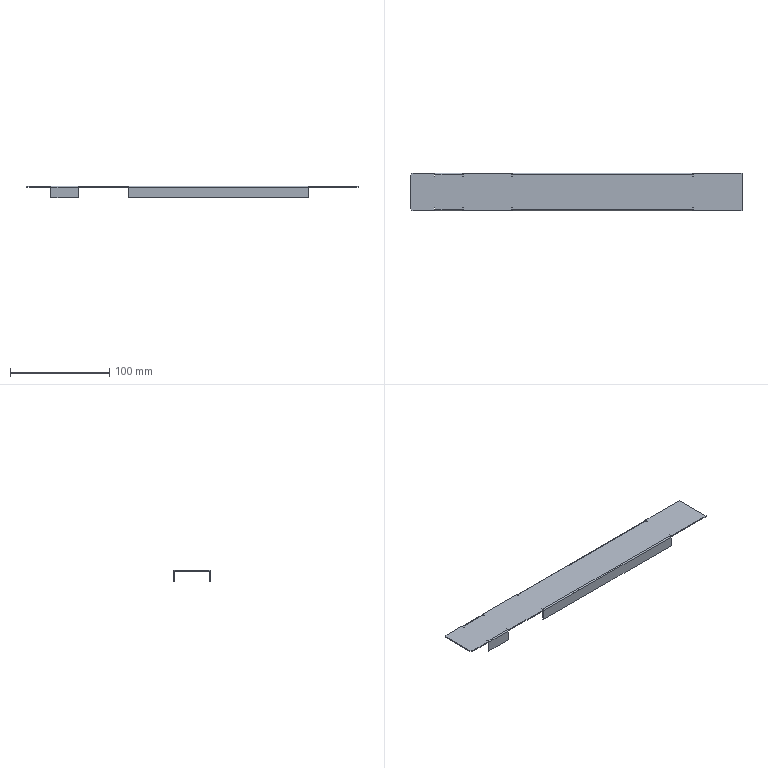Part | 1 solid | 72 faces | box 334.5 x 38 x 12 mm | volume 17189 mm3 | plane 64 | cylinder 8 | commonest cylinder face diameters 0.4 x4 2.4 x4